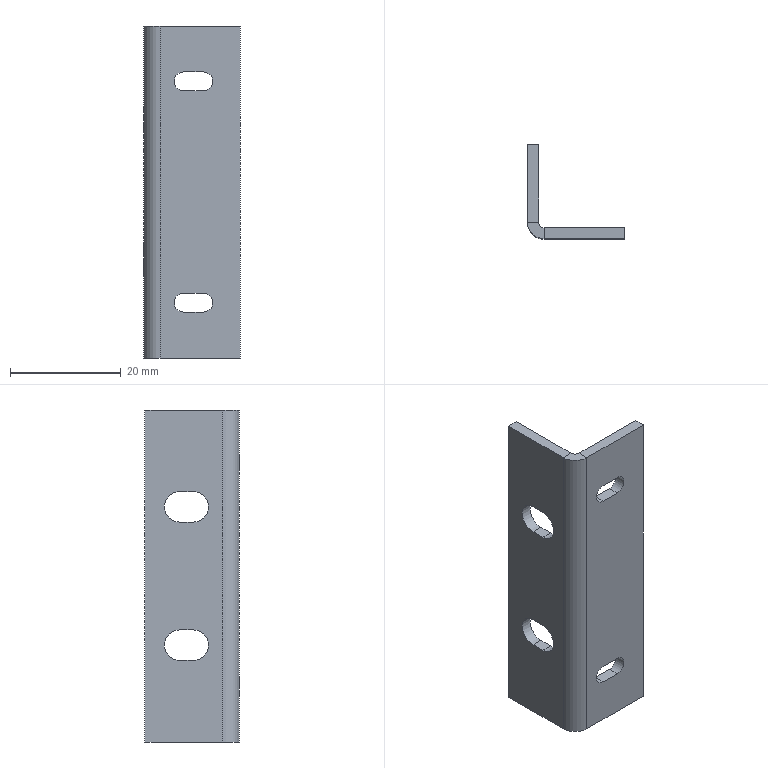Part | SolidWorks | features HoleWzd 2, FlatPattern 1, SMBaseFlange 1, SheetMetal 1 | 1 solid | 30 faces | box 17.5 x 17 x 60 mm | volume 3562 mm3 | plane 20 | cylinder 10 | commonest cylinder face diameters 3.4 x4 5.5 x4 2 x1 6 x1
STEP:
#1=CARTESIAN_POINT('',(0.,-14.,60.));
#2=VERTEX_POINT('',#1);
#3=CARTESIAN_POINT('',(2.,-14.,60.));
#4=VERTEX_POINT('',#3);
#5=CARTESIAN_POINT('',(0.,-14.,60.));
#6=DIRECTION('',(1.,0.,0.));
#7=VECTOR('',#6,1000.);
#8=LINE('',#5,#7);
#9=EDGE_CURVE('',#2,#4,#8,.T.);
#10=ORIENTED_EDGE('',*,*,#9,.F.);
#11=CARTESIAN_POINT('',(3.,-17.,60.));
#12=VERTEX_POINT('',#11);
#13=CARTESIAN_POINT('',(3.,-14.,60.));
#14=DIRECTION('',(0.,0.,1.));
#15=DIRECTION('',(-1.,0.,0.));
#16=AXIS2_PLACEMENT_3D('',#13,#14,#15);
#17=CIRCLE('',#16,3.);
#18=EDGE_CURVE('',#2,#12,#17,.T.);
#19=ORIENTED_EDGE('',*,*,#18,.T.);
#20=CARTESIAN_POINT('',(3.,-15.,60.));
#21=VERTEX_POINT('',#20);
#22=CARTESIAN_POINT('',(3.,-15.,60.));
#23=DIRECTION('',(0.,-1.,0.));
#24=VECTOR('',#23,1000.);
#25=LINE('',#22,#24);
#26=EDGE_CURVE('',#21,#12,#25,.T.);
#27=ORIENTED_EDGE('',*,*,#26,.F.);
#28=CARTESIAN_POINT('',(3.,-14.,60.));
#29=DIRECTION('',(0.,0.,1.));
#30=DIRECTION('',(1.,0.,0.));
#31=AXIS2_PLACEMENT_3D('',#28,#29,#30);
#32=CIRCLE('',#31,1.);
#33=EDGE_CURVE('',#4,#21,#32,.T.);
#34=ORIENTED_EDGE('',*,*,#33,.F.);
#35=EDGE_LOOP('',(#10,#19,#27,#34));
#36=FACE_OUTER_BOUND('',#35,.T.);
#37=CARTESIAN_POINT('',(0.,-14.,60.));
#38=DIRECTION('',(0.,0.,1.));
#39=DIRECTION('',(1.,0.,0.));
#40=AXIS2_PLACEMENT_3D('',#37,#38,#39);
#41=PLANE('',#40);
#42=ADVANCED_FACE('',(#36),#41,.T.);
#43=CARTESIAN_POINT('',(0.,0.,60.));
#44=VERTEX_POINT('',#43);
#45=CARTESIAN_POINT('',(0.,0.,60.));
#46=DIRECTION('',(0.,-1.,0.));
#47=VECTOR('',#46,1000.);
#48=LINE('',#45,#47);
#49=EDGE_CURVE('',#44,#2,#48,.T.);
#50=ORIENTED_EDGE('',*,*,#49,.T.);
#51=ORIENTED_EDGE('',*,*,#9,.T.);
#52=CARTESIAN_POINT('',(2.,0.,60.));
#53=VERTEX_POINT('',#52);
#54=CARTESIAN_POINT('',(2.,0.,60.));
#55=DIRECTION('',(0.,-1.,0.));
#56=VECTOR('',#55,1000.);
#57=LINE('',#54,#56);
#58=EDGE_CURVE('',#53,#4,#57,.T.);
#59=ORIENTED_EDGE('',*,*,#58,.F.);
#60=CARTESIAN_POINT('',(0.,0.,60.));
#61=DIRECTION('',(1.,0.,0.));
#62=VECTOR('',#61,1000.);
#63=LINE('',#60,#62);
#64=EDGE_CURVE('',#44,#53,#63,.T.);
#65=ORIENTED_EDGE('',*,*,#64,.F.);
#66=EDGE_LOOP('',(#50,#51,#59,#65));
#67=FACE_OUTER_BOUND('',#66,.T.);
#68=CARTESIAN_POINT('',(3.,-15.,60.));
#69=DIRECTION('',(0.,0.,1.));
#70=DIRECTION('',(1.,0.,0.));
#71=AXIS2_PLACEMENT_3D('',#68,#69,#70);
#72=PLANE('',#71);
#73=ADVANCED_FACE('',(#67),#72,.T.);
#74=CARTESIAN_POINT('',(3.,-17.,0.));
#75=VERTEX_POINT('',#74);
#76=CARTESIAN_POINT('',(3.,-15.,0.));
#77=VERTEX_POINT('',#76);
#78=CARTESIAN_POINT('',(3.,-17.,0.));
#79=DIRECTION('',(0.,1.,0.));
#80=VECTOR('',#79,1000.);
#81=LINE('',#78,#80);
#82=EDGE_CURVE('',#75,#77,#81,.T.);
#83=ORIENTED_EDGE('',*,*,#82,.F.);
#84=CARTESIAN_POINT('',(0.,-14.,0.));
#85=VERTEX_POINT('',#84);
#86=CARTESIAN_POINT('',(3.,-14.,0.));
#87=DIRECTION('',(0.,0.,1.));
#88=DIRECTION('',(-1.,0.,0.));
#89=AXIS2_PLACEMENT_3D('',#86,#87,#88);
#90=CIRCLE('',#89,3.);
#91=EDGE_CURVE('',#85,#75,#90,.T.);
#92=ORIENTED_EDGE('',*,*,#91,.F.);
#93=CARTESIAN_POINT('',(2.,-14.,0.));
#94=VERTEX_POINT('',#93);
#95=CARTESIAN_POINT('',(2.,-14.,0.));
#96=DIRECTION('',(-1.,0.,0.));
#97=VECTOR('',#96,1000.);
#98=LINE('',#95,#97);
#99=EDGE_CURVE('',#94,#85,#98,.T.);
#100=ORIENTED_EDGE('',*,*,#99,.F.);
#101=CARTESIAN_POINT('',(3.,-14.,0.));
#102=DIRECTION('',(0.,0.,1.));
#103=DIRECTION('',(1.,0.,0.));
#104=AXIS2_PLACEMENT_3D('',#101,#102,#103);
#105=CIRCLE('',#104,1.);
#106=EDGE_CURVE('',#94,#77,#105,.T.);
#107=ORIENTED_EDGE('',*,*,#106,.T.);
#108=EDGE_LOOP('',(#83,#92,#100,#107));
#109=FACE_OUTER_BOUND('',#108,.T.);
#110=CARTESIAN_POINT('',(3.,-17.,0.));
#111=DIRECTION('',(0.,0.,-1.));
#112=DIRECTION('',(-1.,0.,0.));
#113=AXIS2_PLACEMENT_3D('',#110,#111,#112);
#114=PLANE('',#113);
#115=ADVANCED_FACE('',(#109),#114,.T.);
#116=CARTESIAN_POINT('',(17.5,-17.,0.));
#117=VERTEX_POINT('',#116);
#118=CARTESIAN_POINT('',(0.,-17.,0.));
#119=DIRECTION('',(1.,0.,0.));
#120=VECTOR('',#119,1000.);
#121=LINE('',#118,#120);
#122=EDGE_CURVE('',#75,#117,#121,.T.);
#123=ORIENTED_EDGE('',*,*,#122,.F.);
#124=ORIENTED_EDGE('',*,*,#82,.T.);
#125=CARTESIAN_POINT('',(17.5,-15.,0.));
#126=VERTEX_POINT('',#125);
#127=CARTESIAN_POINT('',(0.,-15.,0.));
#128=DIRECTION('',(1.,0.,0.));
#129=VECTOR('',#128,1000.);
#130=LINE('',#127,#129);
#131=EDGE_CURVE('',#77,#126,#130,.T.);
#132=ORIENTED_EDGE('',*,*,#131,.T.);
#133=CARTESIAN_POINT('',(17.5,-15.,0.));
#134=DIRECTION('',(0.,-1.,0.));
#135=VECTOR('',#134,1000.);
#136=LINE('',#133,#135);
#137=EDGE_CURVE('',#126,#117,#136,.T.);
#138=ORIENTED_EDGE('',*,*,#137,.T.);
#139=EDGE_LOOP('',(#123,#124,#132,#138));
#140=FACE_OUTER_BOUND('',#139,.T.);
#141=CARTESIAN_POINT('',(2.,-14.,0.));
#142=DIRECTION('',(0.,0.,-1.));
#143=DIRECTION('',(-1.,0.,0.));
#144=AXIS2_PLACEMENT_3D('',#141,#142,#143);
#145=PLANE('',#144);
#146=ADVANCED_FACE('',(#140),#145,.T.);
#147=CARTESIAN_POINT('',(10.8,-17.,8.3));
#148=VERTEX_POINT('',#147);
#149=CARTESIAN_POINT('',(7.2,-17.,8.3));
#150=VERTEX_POINT('',#149);
#151=CARTESIAN_POINT('',(0.,-17.,8.3));
#152=DIRECTION('',(-1.,0.,0.));
#153=VECTOR('',#152,1000.);
#154=LINE('',#151,#153);
#155=EDGE_CURVE('',#148,#150,#154,.T.);
#156=ORIENTED_EDGE('',*,*,#155,.T.);
#157=CARTESIAN_POINT('',(7.2,-17.,11.7));
#158=VERTEX_POINT('',#157);
#159=CARTESIAN_POINT('',(7.2,-17.,10.));
#160=DIRECTION('',(0.,1.,0.));
#161=DIRECTION('',(0.,0.,1.));
#162=AXIS2_PLACEMENT_3D('',#159,#160,#161);
#163=CIRCLE('',#162,1.7);
#164=EDGE_CURVE('',#150,#158,#163,.T.);
#165=ORIENTED_EDGE('',*,*,#164,.T.);
#166=CARTESIAN_POINT('',(10.8,-17.,11.7));
#167=VERTEX_POINT('',#166);
#168=CARTESIAN_POINT('',(0.,-17.,11.7));
#169=DIRECTION('',(1.,0.,0.));
#170=VECTOR('',#169,1000.);
#171=LINE('',#168,#170);
#172=EDGE_CURVE('',#158,#167,#171,.T.);
#173=ORIENTED_EDGE('',*,*,#172,.T.);
#174=CARTESIAN_POINT('',(10.8,-17.,10.));
#175=DIRECTION('',(0.,1.,0.));
#176=DIRECTION('',(0.,0.,1.));
#177=AXIS2_PLACEMENT_3D('',#174,#175,#176);
#178=CIRCLE('',#177,1.7);
#179=EDGE_CURVE('',#167,#148,#178,.T.);
#180=ORIENTED_EDGE('',*,*,#179,.T.);
#181=EDGE_LOOP('',(#156,#165,#173,#180));
#182=FACE_BOUND('',#181,.T.);
#183=CARTESIAN_POINT('',(10.8,-17.,48.3));
#184=VERTEX_POINT('',#183);
#185=CARTESIAN_POINT('',(7.2,-17.,48.3));
#186=VERTEX_POINT('',#185);
#187=CARTESIAN_POINT('',(0.,-17.,48.3));
#188=DIRECTION('',(-1.,0.,0.));
#189=VECTOR('',#188,1000.);
#190=LINE('',#187,#189);
#191=EDGE_CURVE('',#184,#186,#190,.T.);
#192=ORIENTED_EDGE('',*,*,#191,.T.);
#193=CARTESIAN_POINT('',(7.2,-17.,51.7));
#194=VERTEX_POINT('',#193);
#195=CARTESIAN_POINT('',(7.2,-17.,50.));
#196=DIRECTION('',(0.,1.,0.));
#197=DIRECTION('',(0.,0.,1.));
#198=AXIS2_PLACEMENT_3D('',#195,#196,#197);
#199=CIRCLE('',#198,1.7);
#200=EDGE_CURVE('',#186,#194,#199,.T.);
#201=ORIENTED_EDGE('',*,*,#200,.T.);
#202=CARTESIAN_POINT('',(10.8,-17.,51.7));
#203=VERTEX_POINT('',#202);
#204=CARTESIAN_POINT('',(0.,-17.,51.7));
#205=DIRECTION('',(1.,0.,0.));
#206=VECTOR('',#205,1000.);
#207=LINE('',#204,#206);
#208=EDGE_CURVE('',#194,#203,#207,.T.);
#209=ORIENTED_EDGE('',*,*,#208,.T.);
#210=CARTESIAN_POINT('',(10.8,-17.,50.));
#211=DIRECTION('',(0.,1.,0.));
#212=DIRECTION('',(0.,0.,1.));
#213=AXIS2_PLACEMENT_3D('',#210,#211,#212);
#214=CIRCLE('',#213,1.7);
#215=EDGE_CURVE('',#203,#184,#214,.T.);
#216=ORIENTED_EDGE('',*,*,#215,.T.);
#217=EDGE_LOOP('',(#192,#201,#209,#216));
#218=FACE_BOUND('',#217,.T.);
#219=ORIENTED_EDGE('',*,*,#122,.T.);
#220=CARTESIAN_POINT('',(17.5,-17.,60.));
#221=VERTEX_POINT('',#220);
#222=CARTESIAN_POINT('',(17.5,-17.,60.));
#223=DIRECTION('',(0.,0.,-1.));
#224=VECTOR('',#223,1000.);
#225=LINE('',#222,#224);
#226=EDGE_CURVE('',#221,#117,#225,.T.);
#227=ORIENTED_EDGE('',*,*,#226,.F.);
#228=CARTESIAN_POINT('',(0.,-17.,60.));
#229=DIRECTION('',(1.,0.,0.));
#230=VECTOR('',#229,1000.);
#231=LINE('',#228,#230);
#232=EDGE_CURVE('',#12,#221,#231,.T.);
#233=ORIENTED_EDGE('',*,*,#232,.F.);
#234=CARTESIAN_POINT('',(3.,-17.,60.));
#235=DIRECTION('',(0.,0.,-1.));
#236=VECTOR('',#235,1000.);
#237=LINE('',#234,#236);
#238=EDGE_CURVE('',#12,#75,#237,.T.);
#239=ORIENTED_EDGE('',*,*,#238,.T.);
#240=EDGE_LOOP('',(#219,#227,#233,#239));
#241=FACE_OUTER_BOUND('',#240,.T.);
#242=CARTESIAN_POINT('',(0.,-17.,60.));
#243=DIRECTION('',(0.,1.,0.));
#244=DIRECTION('',(0.,0.,1.));
#245=AXIS2_PLACEMENT_3D('',#242,#243,#244);
#246=PLANE('',#245);
#247=ADVANCED_FACE('',(#182,#218,#241),#246,.F.);
#248=ORIENTED_EDGE('',*,*,#137,.F.);
#249=CARTESIAN_POINT('',(17.5,-15.,60.));
#250=VERTEX_POINT('',#249);
#251=CARTESIAN_POINT('',(17.5,-15.,60.));
#252=DIRECTION('',(0.,0.,-1.));
#253=VECTOR('',#252,1000.);
#254=LINE('',#251,#253);
#255=EDGE_CURVE('',#250,#126,#254,.T.);
#256=ORIENTED_EDGE('',*,*,#255,.F.);
#257=CARTESIAN_POINT('',(17.5,-15.,60.));
#258=DIRECTION('',(0.,-1.,0.));
#259=VECTOR('',#258,1000.);
#260=LINE('',#257,#259);
#261=EDGE_CURVE('',#250,#221,#260,.T.);
#262=ORIENTED_EDGE('',*,*,#261,.T.);
#263=ORIENTED_EDGE('',*,*,#226,.T.);
#264=EDGE_LOOP('',(#248,#256,#262,#263));
#265=FACE_OUTER_BOUND('',#264,.T.);
#266=CARTESIAN_POINT('',(17.5,-15.,60.));
#267=DIRECTION('',(1.,0.,0.));
#268=DIRECTION('',(0.,0.,-1.));
#269=AXIS2_PLACEMENT_3D('',#266,#267,#268);
#270=PLANE('',#269);
#271=ADVANCED_FACE('',(#265),#270,.T.);
#272=CARTESIAN_POINT('',(10.8,-15.,11.7));
#273=VERTEX_POINT('',#272);
#274=CARTESIAN_POINT('',(10.8,-15.,8.3));
#275=VERTEX_POINT('',#274);
#276=CARTESIAN_POINT('',(10.8,-15.,10.));
#277=DIRECTION('',(0.,1.,0.));
#278=DIRECTION('',(0.,0.,1.));
#279=AXIS2_PLACEMENT_3D('',#276,#277,#278);
#280=CIRCLE('',#279,1.7);
#281=EDGE_CURVE('',#273,#275,#280,.T.);
#282=ORIENTED_EDGE('',*,*,#281,.F.);
#283=CARTESIAN_POINT('',(7.2,-15.,11.7));
#284=VERTEX_POINT('',#283);
#285=CARTESIAN_POINT('',(7.2,-15.,11.7));
#286=DIRECTION('',(1.,0.,0.));
#287=VECTOR('',#286,1000.);
#288=LINE('',#285,#287);
#289=EDGE_CURVE('',#284,#273,#288,.T.);
#290=ORIENTED_EDGE('',*,*,#289,.F.);
#291=CARTESIAN_POINT('',(7.2,-15.,8.3));
#292=VERTEX_POINT('',#291);
#293=CARTESIAN_POINT('',(7.2,-15.,10.));
#294=DIRECTION('',(0.,1.,0.));
#295=DIRECTION('',(0.,0.,1.));
#296=AXIS2_PLACEMENT_3D('',#293,#294,#295);
#297=CIRCLE('',#296,1.7);
#298=EDGE_CURVE('',#292,#284,#297,.T.);
#299=ORIENTED_EDGE('',*,*,#298,.F.);
#300=CARTESIAN_POINT('',(7.2,-15.,8.3));
#301=DIRECTION('',(1.,0.,0.));
#302=VECTOR('',#301,1000.);
#303=LINE('',#300,#302);
#304=EDGE_CURVE('',#292,#275,#303,.T.);
#305=ORIENTED_EDGE('',*,*,#304,.T.);
#306=EDGE_LOOP('',(#282,#290,#299,#305));
#307=FACE_BOUND('',#306,.T.);
#308=CARTESIAN_POINT('',(7.2,-15.,51.7));
#309=VERTEX_POINT('',#308);
#310=CARTESIAN_POINT('',(10.8,-15.,51.7));
#311=VERTEX_POINT('',#310);
#312=CARTESIAN_POINT('',(7.2,-15.,51.7));
#313=DIRECTION('',(1.,0.,0.));
#314=VECTOR('',#313,1000.);
#315=LINE('',#312,#314);
#316=EDGE_CURVE('',#309,#311,#315,.T.);
#317=ORIENTED_EDGE('',*,*,#316,.F.);
#318=CARTESIAN_POINT('',(7.2,-15.,48.3));
#319=VERTEX_POINT('',#318);
#320=CARTESIAN_POINT('',(7.2,-15.,50.));
#321=DIRECTION('',(0.,1.,0.));
#322=DIRECTION('',(0.,0.,1.));
#323=AXIS2_PLACEMENT_3D('',#320,#321,#322);
#324=CIRCLE('',#323,1.7);
#325=EDGE_CURVE('',#319,#309,#324,.T.);
#326=ORIENTED_EDGE('',*,*,#325,.F.);
#327=CARTESIAN_POINT('',(10.8,-15.,48.3));
#328=VERTEX_POINT('',#327);
#329=CARTESIAN_POINT('',(7.2,-15.,48.3));
#330=DIRECTION('',(1.,0.,0.));
#331=VECTOR('',#330,1000.);
#332=LINE('',#329,#331);
#333=EDGE_CURVE('',#319,#328,#332,.T.);
#334=ORIENTED_EDGE('',*,*,#333,.T.);
#335=CARTESIAN_POINT('',(10.8,-15.,50.));
#336=DIRECTION('',(0.,1.,0.));
#337=DIRECTION('',(0.,0.,1.));
#338=AXIS2_PLACEMENT_3D('',#335,#336,#337);
#339=CIRCLE('',#338,1.7);
#340=EDGE_CURVE('',#311,#328,#339,.T.);
#341=ORIENTED_EDGE('',*,*,#340,.F.);
#342=EDGE_LOOP('',(#317,#326,#334,#341));
#343=FACE_BOUND('',#342,.T.);
#344=ORIENTED_EDGE('',*,*,#131,.F.);
#345=CARTESIAN_POINT('',(3.,-15.,60.));
#346=DIRECTION('',(0.,0.,-1.));
#347=VECTOR('',#346,1000.);
#348=LINE('',#345,#347);
#349=EDGE_CURVE('',#21,#77,#348,.T.);
#350=ORIENTED_EDGE('',*,*,#349,.F.);
#351=CARTESIAN_POINT('',(0.,-15.,60.));
#352=DIRECTION('',(1.,0.,0.));
#353=VECTOR('',#352,1000.);
#354=LINE('',#351,#353);
#355=EDGE_CURVE('',#21,#250,#354,.T.);
#356=ORIENTED_EDGE('',*,*,#355,.T.);
#357=ORIENTED_EDGE('',*,*,#255,.T.);
#358=EDGE_LOOP('',(#344,#350,#356,#357));
#359=FACE_OUTER_BOUND('',#358,.T.);
#360=CARTESIAN_POINT('',(0.,-15.,60.));
#361=DIRECTION('',(0.,1.,0.));
#362=DIRECTION('',(0.,0.,1.));
#363=AXIS2_PLACEMENT_3D('',#360,#361,#362);
#364=PLANE('',#363);
#365=ADVANCED_FACE('',(#307,#343,#359),#364,.T.);
#366=ORIENTED_EDGE('',*,*,#106,.F.);
#367=CARTESIAN_POINT('',(2.,-14.,60.));
#368=DIRECTION('',(0.,0.,-1.));
#369=VECTOR('',#368,1000.);
#370=LINE('',#367,#369);
#371=EDGE_CURVE('',#4,#94,#370,.T.);
#372=ORIENTED_EDGE('',*,*,#371,.F.);
#373=ORIENTED_EDGE('',*,*,#33,.T.);
#374=ORIENTED_EDGE('',*,*,#349,.T.);
#375=EDGE_LOOP('',(#366,#372,#373,#374));
#376=FACE_OUTER_BOUND('',#375,.T.);
#377=CARTESIAN_POINT('',(3.,-14.,60.));
#378=DIRECTION('',(0.,0.,-1.));
#379=DIRECTION('',(-1.,0.,0.));
#380=AXIS2_PLACEMENT_3D('',#377,#378,#379);
#381=CYLINDRICAL_SURFACE('',#380,1.);
#382=ADVANCED_FACE('',(#376),#381,.F.);
#383=CARTESIAN_POINT('',(2.,-6.25,14.75));
#384=VERTEX_POINT('',#383);
#385=CARTESIAN_POINT('',(2.,-6.25,20.25));
#386=VERTEX_POINT('',#385);
#387=CARTESIAN_POINT('',(2.,-6.25,17.5));
#388=DIRECTION('',(1.,0.,0.));
#389=DIRECTION('',(0.,0.,-1.));
#390=AXIS2_PLACEMENT_3D('',#387,#388,#389);
#391=CIRCLE('',#390,2.75);
#392=EDGE_CURVE('',#384,#386,#391,.T.);
#393=ORIENTED_EDGE('',*,*,#392,.F.);
#394=CARTESIAN_POINT('',(2.,-8.75,14.75));
#395=VERTEX_POINT('',#394);
#396=CARTESIAN_POINT('',(2.,-8.75,14.75));
#397=DIRECTION('',(0.,1.,0.));
#398=VECTOR('',#397,1000.);
#399=LINE('',#396,#398);
#400=EDGE_CURVE('',#395,#384,#399,.T.);
#401=ORIENTED_EDGE('',*,*,#400,.F.);
#402=CARTESIAN_POINT('',(2.,-8.75,20.25));
#403=VERTEX_POINT('',#402);
#404=CARTESIAN_POINT('',(2.,-8.75,17.5));
#405=DIRECTION('',(1.,0.,0.));
#406=DIRECTION('',(0.,0.,-1.));
#407=AXIS2_PLACEMENT_3D('',#404,#405,#406);
#408=CIRCLE('',#407,2.75);
#409=EDGE_CURVE('',#403,#395,#408,.T.);
#410=ORIENTED_EDGE('',*,*,#409,.F.);
#411=CARTESIAN_POINT('',(2.,-8.75,20.25));
#412=DIRECTION('',(0.,1.,0.));
#413=VECTOR('',#412,1000.);
#414=LINE('',#411,#413);
#415=EDGE_CURVE('',#403,#386,#414,.T.);
#416=ORIENTED_EDGE('',*,*,#415,.T.);
#417=EDGE_LOOP('',(#393,#401,#410,#416));
#418=FACE_BOUND('',#417,.T.);
#419=CARTESIAN_POINT('',(2.,-8.75,39.75));
#420=VERTEX_POINT('',#419);
#421=CARTESIAN_POINT('',(2.,-6.25,39.75));
#422=VERTEX_POINT('',#421);
#423=CARTESIAN_POINT('',(2.,-8.75,39.75));
#424=DIRECTION('',(0.,1.,0.));
#425=VECTOR('',#424,1000.);
#426=LINE('',#423,#425);
#427=EDGE_CURVE('',#420,#422,#426,.T.);
#428=ORIENTED_EDGE('',*,*,#427,.F.);
#429=CARTESIAN_POINT('',(2.,-8.75,45.25));
#430=VERTEX_POINT('',#429);
#431=CARTESIAN_POINT('',(2.,-8.75,42.5));
#432=DIRECTION('',(1.,0.,0.));
#433=DIRECTION('',(0.,0.,-1.));
#434=AXIS2_PLACEMENT_3D('',#431,#432,#433);
#435=CIRCLE('',#434,2.75);
#436=EDGE_CURVE('',#430,#420,#435,.T.);
#437=ORIENTED_EDGE('',*,*,#436,.F.);
#438=CARTESIAN_POINT('',(2.,-6.25,45.25));
#439=VERTEX_POINT('',#438);
#440=CARTESIAN_POINT('',(2.,-8.75,45.25));
#441=DIRECTION('',(0.,1.,0.));
#442=VECTOR('',#441,1000.);
#443=LINE('',#440,#442);
#444=EDGE_CURVE('',#430,#439,#443,.T.);
#445=ORIENTED_EDGE('',*,*,#444,.T.);
#446=CARTESIAN_POINT('',(2.,-6.25,42.5));
#447=DIRECTION('',(1.,0.,0.));
#448=DIRECTION('',(0.,0.,-1.));
#449=AXIS2_PLACEMENT_3D('',#446,#447,#448);
#450=CIRCLE('',#449,2.75);
#451=EDGE_CURVE('',#422,#439,#450,.T.);
#452=ORIENTED_EDGE('',*,*,#451,.F.);
#453=EDGE_LOOP('',(#428,#437,#445,#452));
#454=FACE_BOUND('',#453,.T.);
#455=CARTESIAN_POINT('',(2.,0.,0.));
#456=VERTEX_POINT('',#455);
#457=CARTESIAN_POINT('',(2.,0.,0.));
#458=DIRECTION('',(0.,-1.,0.));
#459=VECTOR('',#458,1000.);
#460=LINE('',#457,#459);
#461=EDGE_CURVE('',#456,#94,#460,.T.);
#462=ORIENTED_EDGE('',*,*,#461,.F.);
#463=CARTESIAN_POINT('',(2.,0.,60.));
#464=DIRECTION('',(0.,0.,-1.));
#465=VECTOR('',#464,1000.);
#466=LINE('',#463,#465);
#467=EDGE_CURVE('',#53,#456,#466,.T.);
#468=ORIENTED_EDGE('',*,*,#467,.F.);
#469=ORIENTED_EDGE('',*,*,#58,.T.);
#470=ORIENTED_EDGE('',*,*,#371,.T.);
#471=EDGE_LOOP('',(#462,#468,#469,#470));
#472=FACE_OUTER_BOUND('',#471,.T.);
#473=CARTESIAN_POINT('',(2.,0.,60.));
#474=DIRECTION('',(1.,0.,0.));
#475=DIRECTION('',(0.,1.,0.));
#476=AXIS2_PLACEMENT_3D('',#473,#474,#475);
#477=PLANE('',#476);
#478=ADVANCED_FACE('',(#418,#454,#472),#477,.T.);
#479=CARTESIAN_POINT('',(0.,0.,0.));
#480=VERTEX_POINT('',#479);
#481=CARTESIAN_POINT('',(0.,0.,0.));
#482=DIRECTION('',(1.,0.,0.));
#483=VECTOR('',#482,1000.);
#484=LINE('',#481,#483);
#485=EDGE_CURVE('',#480,#456,#484,.T.);
#486=ORIENTED_EDGE('',*,*,#485,.F.);
#487=CARTESIAN_POINT('',(0.,0.,60.));
#488=DIRECTION('',(0.,0.,-1.));
#489=VECTOR('',#488,1000.);
#490=LINE('',#487,#489);
#491=EDGE_CURVE('',#44,#480,#490,.T.);
#492=ORIENTED_EDGE('',*,*,#491,.F.);
#493=ORIENTED_EDGE('',*,*,#64,.T.);
#494=ORIENTED_EDGE('',*,*,#467,.T.);
#495=EDGE_LOOP('',(#486,#492,#493,#494));
#496=FACE_OUTER_BOUND('',#495,.T.);
#497=CARTESIAN_POINT('',(0.,0.,60.));
#498=DIRECTION('',(0.,1.,0.));
#499=DIRECTION('',(-1.,0.,0.));
#500=AXIS2_PLACEMENT_3D('',#497,#498,#499);
#501=PLANE('',#500);
#502=ADVANCED_FACE('',(#496),#501,.T.);
#503=CARTESIAN_POINT('',(0.,-6.25,20.25));
#504=VERTEX_POINT('',#503);
#505=CARTESIAN_POINT('',(0.,-8.75,20.25));
#506=VERTEX_POINT('',#505);
#507=CARTESIAN_POINT('',(0.,0.,20.25));
#508=DIRECTION('',(0.,-1.,0.));
#509=VECTOR('',#508,1000.);
#510=LINE('',#507,#509);
#511=EDGE_CURVE('',#504,#506,#510,.T.);
#512=ORIENTED_EDGE('',*,*,#511,.T.);
#513=CARTESIAN_POINT('',(0.,-8.75,14.75));
#514=VERTEX_POINT('',#513);
#515=CARTESIAN_POINT('',(0.,-8.75,17.5));
#516=DIRECTION('',(1.,0.,0.));
#517=DIRECTION('',(0.,1.,0.));
#518=AXIS2_PLACEMENT_3D('',#515,#516,#517);
#519=CIRCLE('',#518,2.75);
#520=EDGE_CURVE('',#506,#514,#519,.T.);
#521=ORIENTED_EDGE('',*,*,#520,.T.);
#522=CARTESIAN_POINT('',(0.,-6.25,14.75));
#523=VERTEX_POINT('',#522);
#524=CARTESIAN_POINT('',(0.,0.,14.75));
#525=DIRECTION('',(0.,1.,0.));
#526=VECTOR('',#525,1000.);
#527=LINE('',#524,#526);
#528=EDGE_CURVE('',#514,#523,#527,.T.);
#529=ORIENTED_EDGE('',*,*,#528,.T.);
#530=CARTESIAN_POINT('',(0.,-6.25,17.5));
#531=DIRECTION('',(1.,0.,0.));
#532=DIRECTION('',(0.,1.,0.));
#533=AXIS2_PLACEMENT_3D('',#530,#531,#532);
#534=CIRCLE('',#533,2.75);
#535=EDGE_CURVE('',#523,#504,#534,.T.);
#536=ORIENTED_EDGE('',*,*,#535,.T.);
#537=EDGE_LOOP('',(#512,#521,#529,#536));
#538=FACE_BOUND('',#537,.T.);
#539=CARTESIAN_POINT('',(0.,-8.75,39.75));
#540=VERTEX_POINT('',#539);
#541=CARTESIAN_POINT('',(0.,-6.25,39.75));
#542=VERTEX_POINT('',#541);
#543=CARTESIAN_POINT('',(0.,0.,39.75));
#544=DIRECTION('',(0.,1.,0.));
#545=VECTOR('',#544,1000.);
#546=LINE('',#543,#545);
#547=EDGE_CURVE('',#540,#542,#546,.T.);
#548=ORIENTED_EDGE('',*,*,#547,.T.);
#549=CARTESIAN_POINT('',(0.,-6.25,45.25));
#550=VERTEX_POINT('',#549);
#551=CARTESIAN_POINT('',(0.,-6.25,42.5));
#552=DIRECTION('',(1.,0.,0.));
#553=DIRECTION('',(0.,1.,0.));
#554=AXIS2_PLACEMENT_3D('',#551,#552,#553);
#555=CIRCLE('',#554,2.75);
#556=EDGE_CURVE('',#542,#550,#555,.T.);
#557=ORIENTED_EDGE('',*,*,#556,.T.);
#558=CARTESIAN_POINT('',(0.,-8.75,45.25));
#559=VERTEX_POINT('',#558);
#560=CARTESIAN_POINT('',(0.,0.,45.25));
#561=DIRECTION('',(0.,-1.,0.));
#562=VECTOR('',#561,1000.);
#563=LINE('',#560,#562);
#564=EDGE_CURVE('',#550,#559,#563,.T.);
#565=ORIENTED_EDGE('',*,*,#564,.T.);
#566=CARTESIAN_POINT('',(0.,-8.75,42.5));
#567=DIRECTION('',(1.,0.,0.));
#568=DIRECTION('',(0.,1.,0.));
#569=AXIS2_PLACEMENT_3D('',#566,#567,#568);
#570=CIRCLE('',#569,2.75);
#571=EDGE_CURVE('',#559,#540,#570,.T.);
#572=ORIENTED_EDGE('',*,*,#571,.T.);
#573=EDGE_LOOP('',(#548,#557,#565,#572));
#574=FACE_BOUND('',#573,.T.);
#575=CARTESIAN_POINT('',(0.,0.,0.));
#576=DIRECTION('',(0.,-1.,0.));
#577=VECTOR('',#576,1000.);
#578=LINE('',#575,#577);
#579=EDGE_CURVE('',#480,#85,#578,.T.);
#580=ORIENTED_EDGE('',*,*,#579,.T.);
#581=CARTESIAN_POINT('',(0.,-14.,60.));
#582=DIRECTION('',(0.,0.,-1.));
#583=VECTOR('',#582,1000.);
#584=LINE('',#581,#583);
#585=EDGE_CURVE('',#2,#85,#584,.T.);
#586=ORIENTED_EDGE('',*,*,#585,.F.);
#587=ORIENTED_EDGE('',*,*,#49,.F.);
#588=ORIENTED_EDGE('',*,*,#491,.T.);
#589=EDGE_LOOP('',(#580,#586,#587,#588));
#590=FACE_OUTER_BOUND('',#589,.T.);
#591=CARTESIAN_POINT('',(0.,0.,60.));
#592=DIRECTION('',(1.,0.,0.));
#593=DIRECTION('',(0.,1.,0.));
#594=AXIS2_PLACEMENT_3D('',#591,#592,#593);
#595=PLANE('',#594);
#596=ADVANCED_FACE('',(#538,#574,#590),#595,.F.);
#597=ORIENTED_EDGE('',*,*,#91,.T.);
#598=ORIENTED_EDGE('',*,*,#238,.F.);
#599=ORIENTED_EDGE('',*,*,#18,.F.);
#600=ORIENTED_EDGE('',*,*,#585,.T.);
#601=EDGE_LOOP('',(#597,#598,#599,#600));
#602=FACE_OUTER_BOUND('',#601,.T.);
#603=CARTESIAN_POINT('',(3.,-14.,60.));
#604=DIRECTION('',(0.,0.,-1.));
#605=DIRECTION('',(-1.,0.,0.));
#606=AXIS2_PLACEMENT_3D('',#603,#604,#605);
#607=CYLINDRICAL_SURFACE('',#606,3.);
#608=ADVANCED_FACE('',(#602),#607,.T.);
#609=ORIENTED_EDGE('',*,*,#232,.T.);
#610=ORIENTED_EDGE('',*,*,#261,.F.);
#611=ORIENTED_EDGE('',*,*,#355,.F.);
#612=ORIENTED_EDGE('',*,*,#26,.T.);
#613=EDGE_LOOP('',(#609,#610,#611,#612));
#614=FACE_OUTER_BOUND('',#613,.T.);
#615=CARTESIAN_POINT('',(3.,-14.,60.));
#616=DIRECTION('',(0.,0.,1.));
#617=DIRECTION('',(1.,0.,0.));
#618=AXIS2_PLACEMENT_3D('',#615,#616,#617);
#619=PLANE('',#618);
#620=ADVANCED_FACE('',(#614),#619,.T.);
#621=ORIENTED_EDGE('',*,*,#461,.T.);
#622=ORIENTED_EDGE('',*,*,#99,.T.);
#623=ORIENTED_EDGE('',*,*,#579,.F.);
#624=ORIENTED_EDGE('',*,*,#485,.T.);
#625=EDGE_LOOP('',(#621,#622,#623,#624));
#626=FACE_OUTER_BOUND('',#625,.T.);
#627=CARTESIAN_POINT('',(3.,-14.,0.));
#628=DIRECTION('',(0.,0.,1.));
#629=DIRECTION('',(1.,0.,0.));
#630=AXIS2_PLACEMENT_3D('',#627,#628,#629);
#631=PLANE('',#630);
#632=ADVANCED_FACE('',(#626),#631,.F.);
#633=CARTESIAN_POINT('',(7.2,-15.,48.3));
#634=DIRECTION('',(0.,-1.,0.));
#635=VECTOR('',#634,1000.);
#636=LINE('',#633,#635);
#637=EDGE_CURVE('',#319,#186,#636,.T.);
#638=ORIENTED_EDGE('',*,*,#637,.F.);
#639=ORIENTED_EDGE('',*,*,#325,.T.);
#640=CARTESIAN_POINT('',(7.2,-15.,51.7));
#641=DIRECTION('',(0.,1.,0.));
#642=VECTOR('',#641,1000.);
#643=LINE('',#640,#642);
#644=EDGE_CURVE('',#194,#309,#643,.T.);
#645=ORIENTED_EDGE('',*,*,#644,.F.);
#646=ORIENTED_EDGE('',*,*,#200,.F.);
#647=EDGE_LOOP('',(#638,#639,#645,#646));
#648=FACE_OUTER_BOUND('',#647,.T.);
#649=CARTESIAN_POINT('',(7.2,-15.,50.));
#650=DIRECTION('',(0.,1.,0.));
#651=DIRECTION('',(0.,0.,1.));
#652=AXIS2_PLACEMENT_3D('',#649,#650,#651);
#653=CYLINDRICAL_SURFACE('',#652,1.7);
#654=ADVANCED_FACE('',(#648),#653,.F.);
#655=ORIENTED_EDGE('',*,*,#644,.T.);
#656=ORIENTED_EDGE('',*,*,#316,.T.);
#657=CARTESIAN_POINT('',(10.8,-15.,51.7));
#658=DIRECTION('',(0.,-1.,0.));
#659=VECTOR('',#658,1000.);
#660=LINE('',#657,#659);
#661=EDGE_CURVE('',#311,#203,#660,.T.);
#662=ORIENTED_EDGE('',*,*,#661,.T.);
#663=ORIENTED_EDGE('',*,*,#208,.F.);
#664=EDGE_LOOP('',(#655,#656,#662,#663));
#665=FACE_OUTER_BOUND('',#664,.T.);
#666=CARTESIAN_POINT('',(7.2,-15.,51.7));
#667=DIRECTION('',(0.,0.,1.));
#668=DIRECTION('',(1.,0.,0.));
#669=AXIS2_PLACEMENT_3D('',#666,#667,#668);
#670=PLANE('',#669);
#671=ADVANCED_FACE('',(#665),#670,.F.);
#672=CARTESIAN_POINT('',(10.8,-15.,48.3));
#673=DIRECTION('',(0.,1.,0.));
#674=VECTOR('',#673,1000.);
#675=LINE('',#672,#674);
#676=EDGE_CURVE('',#184,#328,#675,.T.);
#677=ORIENTED_EDGE('',*,*,#676,.T.);
#678=ORIENTED_EDGE('',*,*,#333,.F.);
#679=ORIENTED_EDGE('',*,*,#637,.T.);
#680=ORIENTED_EDGE('',*,*,#191,.F.);
#681=EDGE_LOOP('',(#677,#678,#679,#680));
#682=FACE_OUTER_BOUND('',#681,.T.);
#683=CARTESIAN_POINT('',(7.2,-15.,48.3));
#684=DIRECTION('',(0.,0.,-1.));
#685=DIRECTION('',(-1.,0.,0.));
#686=AXIS2_PLACEMENT_3D('',#683,#684,#685);
#687=PLANE('',#686);
#688=ADVANCED_FACE('',(#682),#687,.F.);
#689=ORIENTED_EDGE('',*,*,#661,.F.);
#690=ORIENTED_EDGE('',*,*,#340,.T.);
#691=ORIENTED_EDGE('',*,*,#676,.F.);
#692=ORIENTED_EDGE('',*,*,#215,.F.);
#693=EDGE_LOOP('',(#689,#690,#691,#692));
#694=FACE_OUTER_BOUND('',#693,.T.);
#695=CARTESIAN_POINT('',(10.8,-15.,50.));
#696=DIRECTION('',(0.,1.,0.));
#697=DIRECTION('',(0.,0.,1.));
#698=AXIS2_PLACEMENT_3D('',#695,#696,#697);
#699=CYLINDRICAL_SURFACE('',#698,1.7);
#700=ADVANCED_FACE('',(#694),#699,.F.);
#701=CARTESIAN_POINT('',(7.2,-15.,8.3));
#702=DIRECTION('',(0.,-1.,0.));
#703=VECTOR('',#702,1000.);
#704=LINE('',#701,#703);
#705=EDGE_CURVE('',#292,#150,#704,.T.);
#706=ORIENTED_EDGE('',*,*,#705,.F.);
#707=ORIENTED_EDGE('',*,*,#298,.T.);
#708=CARTESIAN_POINT('',(7.2,-15.,11.7));
#709=DIRECTION('',(0.,1.,0.));
#710=VECTOR('',#709,1000.);
#711=LINE('',#708,#710);
#712=EDGE_CURVE('',#158,#284,#711,.T.);
#713=ORIENTED_EDGE('',*,*,#712,.F.);
#714=ORIENTED_EDGE('',*,*,#164,.F.);
#715=EDGE_LOOP('',(#706,#707,#713,#714));
#716=FACE_OUTER_BOUND('',#715,.T.);
#717=CARTESIAN_POINT('',(7.2,-15.,10.));
#718=DIRECTION('',(0.,1.,0.));
#719=DIRECTION('',(0.,0.,1.));
#720=AXIS2_PLACEMENT_3D('',#717,#718,#719);
#721=CYLINDRICAL_SURFACE('',#720,1.7);
#722=ADVANCED_FACE('',(#716),#721,.F.);
#723=ORIENTED_EDGE('',*,*,#712,.T.);
#724=ORIENTED_EDGE('',*,*,#289,.T.);
#725=CARTESIAN_POINT('',(10.8,-15.,11.7));
#726=DIRECTION('',(0.,-1.,0.));
#727=VECTOR('',#726,1000.);
#728=LINE('',#725,#727);
#729=EDGE_CURVE('',#273,#167,#728,.T.);
#730=ORIENTED_EDGE('',*,*,#729,.T.);
#731=ORIENTED_EDGE('',*,*,#172,.F.);
#732=EDGE_LOOP('',(#723,#724,#730,#731));
#733=FACE_OUTER_BOUND('',#732,.T.);
#734=CARTESIAN_POINT('',(7.2,-15.,11.7));
#735=DIRECTION('',(0.,0.,1.));
#736=DIRECTION('',(1.,0.,0.));
#737=AXIS2_PLACEMENT_3D('',#734,#735,#736);
#738=PLANE('',#737);
#739=ADVANCED_FACE('',(#733),#738,.F.);
#740=ORIENTED_EDGE('',*,*,#729,.F.);
#741=ORIENTED_EDGE('',*,*,#281,.T.);
#742=CARTESIAN_POINT('',(10.8,-15.,8.3));
#743=DIRECTION('',(0.,1.,0.));
#744=VECTOR('',#743,1000.);
#745=LINE('',#742,#744);
#746=EDGE_CURVE('',#148,#275,#745,.T.);
#747=ORIENTED_EDGE('',*,*,#746,.F.);
#748=ORIENTED_EDGE('',*,*,#179,.F.);
#749=EDGE_LOOP('',(#740,#741,#747,#748));
#750=FACE_OUTER_BOUND('',#749,.T.);
#751=CARTESIAN_POINT('',(10.8,-15.,10.));
#752=DIRECTION('',(0.,1.,0.));
#753=DIRECTION('',(0.,0.,1.));
#754=AXIS2_PLACEMENT_3D('',#751,#752,#753);
#755=CYLINDRICAL_SURFACE('',#754,1.7);
#756=ADVANCED_FACE('',(#750),#755,.F.);
#757=ORIENTED_EDGE('',*,*,#746,.T.);
#758=ORIENTED_EDGE('',*,*,#304,.F.);
#759=ORIENTED_EDGE('',*,*,#705,.T.);
#760=ORIENTED_EDGE('',*,*,#155,.F.);
#761=EDGE_LOOP('',(#757,#758,#759,#760));
#762=FACE_OUTER_BOUND('',#761,.T.);
#763=CARTESIAN_POINT('',(7.2,-15.,8.3));
#764=DIRECTION('',(0.,0.,-1.));
#765=DIRECTION('',(-1.,0.,0.));
#766=AXIS2_PLACEMENT_3D('',#763,#764,#765);
#767=PLANE('',#766);
#768=ADVANCED_FACE('',(#762),#767,.F.);
#769=CARTESIAN_POINT('',(2.,-6.25,39.75));
#770=DIRECTION('',(-1.,0.,0.));
#771=VECTOR('',#770,1000.);
#772=LINE('',#769,#771);
#773=EDGE_CURVE('',#422,#542,#772,.T.);
#774=ORIENTED_EDGE('',*,*,#773,.F.);
#775=ORIENTED_EDGE('',*,*,#451,.T.);
#776=CARTESIAN_POINT('',(2.,-6.25,45.25));
#777=DIRECTION('',(1.,0.,0.));
#778=VECTOR('',#777,1000.);
#779=LINE('',#776,#778);
#780=EDGE_CURVE('',#550,#439,#779,.T.);
#781=ORIENTED_EDGE('',*,*,#780,.F.);
#782=ORIENTED_EDGE('',*,*,#556,.F.);
#783=EDGE_LOOP('',(#774,#775,#781,#782));
#784=FACE_OUTER_BOUND('',#783,.T.);
#785=CARTESIAN_POINT('',(2.,-6.25,42.5));
#786=DIRECTION('',(1.,0.,0.));
#787=DIRECTION('',(0.,0.,-1.));
#788=AXIS2_PLACEMENT_3D('',#785,#786,#787);
#789=CYLINDRICAL_SURFACE('',#788,2.75);
#790=ADVANCED_FACE('',(#784),#789,.F.);
#791=CARTESIAN_POINT('',(2.,-8.75,39.75));
#792=DIRECTION('',(1.,0.,0.));
#793=VECTOR('',#792,1000.);
#794=LINE('',#791,#793);
#795=EDGE_CURVE('',#540,#420,#794,.T.);
#796=ORIENTED_EDGE('',*,*,#795,.T.);
#797=ORIENTED_EDGE('',*,*,#427,.T.);
#798=ORIENTED_EDGE('',*,*,#773,.T.);
#799=ORIENTED_EDGE('',*,*,#547,.F.);
#800=EDGE_LOOP('',(#796,#797,#798,#799));
#801=FACE_OUTER_BOUND('',#800,.T.);
#802=CARTESIAN_POINT('',(2.,-8.75,39.75));
#803=DIRECTION('',(0.,0.,-1.));
#804=DIRECTION('',(-1.,0.,0.));
#805=AXIS2_PLACEMENT_3D('',#802,#803,#804);
#806=PLANE('',#805);
#807=ADVANCED_FACE('',(#801),#806,.F.);
#808=ORIENTED_EDGE('',*,*,#780,.T.);
#809=ORIENTED_EDGE('',*,*,#444,.F.);
#810=CARTESIAN_POINT('',(2.,-8.75,45.25));
#811=DIRECTION('',(-1.,0.,0.));
#812=VECTOR('',#811,1000.);
#813=LINE('',#810,#812);
#814=EDGE_CURVE('',#430,#559,#813,.T.);
#815=ORIENTED_EDGE('',*,*,#814,.T.);
#816=ORIENTED_EDGE('',*,*,#564,.F.);
#817=EDGE_LOOP('',(#808,#809,#815,#816));
#818=FACE_OUTER_BOUND('',#817,.T.);
#819=CARTESIAN_POINT('',(2.,-8.75,45.25));
#820=DIRECTION('',(0.,0.,1.));
#821=DIRECTION('',(1.,0.,0.));
#822=AXIS2_PLACEMENT_3D('',#819,#820,#821);
#823=PLANE('',#822);
#824=ADVANCED_FACE('',(#818),#823,.F.);
#825=ORIENTED_EDGE('',*,*,#814,.F.);
#826=ORIENTED_EDGE('',*,*,#436,.T.);
#827=ORIENTED_EDGE('',*,*,#795,.F.);
#828=ORIENTED_EDGE('',*,*,#571,.F.);
#829=EDGE_LOOP('',(#825,#826,#827,#828));
#830=FACE_OUTER_BOUND('',#829,.T.);
#831=CARTESIAN_POINT('',(2.,-8.75,42.5));
#832=DIRECTION('',(1.,0.,0.));
#833=DIRECTION('',(0.,0.,-1.));
#834=AXIS2_PLACEMENT_3D('',#831,#832,#833);
#835=CYLINDRICAL_SURFACE('',#834,2.75);
#836=ADVANCED_FACE('',(#830),#835,.F.);
#837=CARTESIAN_POINT('',(2.,-8.75,20.25));
#838=DIRECTION('',(-1.,0.,0.));
#839=VECTOR('',#838,1000.);
#840=LINE('',#837,#839);
#841=EDGE_CURVE('',#403,#506,#840,.T.);
#842=ORIENTED_EDGE('',*,*,#841,.F.);
#843=ORIENTED_EDGE('',*,*,#409,.T.);
#844=CARTESIAN_POINT('',(2.,-8.75,14.75));
#845=DIRECTION('',(1.,0.,0.));
#846=VECTOR('',#845,1000.);
#847=LINE('',#844,#846);
#848=EDGE_CURVE('',#514,#395,#847,.T.);
#849=ORIENTED_EDGE('',*,*,#848,.F.);
#850=ORIENTED_EDGE('',*,*,#520,.F.);
#851=EDGE_LOOP('',(#842,#843,#849,#850));
#852=FACE_OUTER_BOUND('',#851,.T.);
#853=CARTESIAN_POINT('',(2.,-8.75,17.5));
#854=DIRECTION('',(1.,0.,0.));
#855=DIRECTION('',(0.,0.,-1.));
#856=AXIS2_PLACEMENT_3D('',#853,#854,#855);
#857=CYLINDRICAL_SURFACE('',#856,2.75);
#858=ADVANCED_FACE('',(#852),#857,.F.);
#859=ORIENTED_EDGE('',*,*,#848,.T.);
#860=ORIENTED_EDGE('',*,*,#400,.T.);
#861=CARTESIAN_POINT('',(2.,-6.25,14.75));
#862=DIRECTION('',(-1.,0.,0.));
#863=VECTOR('',#862,1000.);
#864=LINE('',#861,#863);
#865=EDGE_CURVE('',#384,#523,#864,.T.);
#866=ORIENTED_EDGE('',*,*,#865,.T.);
#867=ORIENTED_EDGE('',*,*,#528,.F.);
#868=EDGE_LOOP('',(#859,#860,#866,#867));
#869=FACE_OUTER_BOUND('',#868,.T.);
#870=CARTESIAN_POINT('',(2.,-8.75,14.75));
#871=DIRECTION('',(0.,0.,-1.));
#872=DIRECTION('',(-1.,0.,0.));
#873=AXIS2_PLACEMENT_3D('',#870,#871,#872);
#874=PLANE('',#873);
#875=ADVANCED_FACE('',(#869),#874,.F.);
#876=CARTESIAN_POINT('',(2.,-6.25,20.25));
#877=DIRECTION('',(1.,0.,0.));
#878=VECTOR('',#877,1000.);
#879=LINE('',#876,#878);
#880=EDGE_CURVE('',#504,#386,#879,.T.);
#881=ORIENTED_EDGE('',*,*,#880,.T.);
#882=ORIENTED_EDGE('',*,*,#415,.F.);
#883=ORIENTED_EDGE('',*,*,#841,.T.);
#884=ORIENTED_EDGE('',*,*,#511,.F.);
#885=EDGE_LOOP('',(#881,#882,#883,#884));
#886=FACE_OUTER_BOUND('',#885,.T.);
#887=CARTESIAN_POINT('',(2.,-8.75,20.25));
#888=DIRECTION('',(0.,0.,1.));
#889=DIRECTION('',(1.,0.,0.));
#890=AXIS2_PLACEMENT_3D('',#887,#888,#889);
#891=PLANE('',#890);
#892=ADVANCED_FACE('',(#886),#891,.F.);
#893=ORIENTED_EDGE('',*,*,#865,.F.);
#894=ORIENTED_EDGE('',*,*,#392,.T.);
#895=ORIENTED_EDGE('',*,*,#880,.F.);
#896=ORIENTED_EDGE('',*,*,#535,.F.);
#897=EDGE_LOOP('',(#893,#894,#895,#896));
#898=FACE_OUTER_BOUND('',#897,.T.);
#899=CARTESIAN_POINT('',(2.,-6.25,17.5));
#900=DIRECTION('',(1.,0.,0.));
#901=DIRECTION('',(0.,0.,-1.));
#902=AXIS2_PLACEMENT_3D('',#899,#900,#901);
#903=CYLINDRICAL_SURFACE('',#902,2.75);
#904=ADVANCED_FACE('',(#898),#903,.F.);
#905=CLOSED_SHELL('',(#42,#73,#115,#146,#247,#271,#365,#382,#478,#502,#596,#608,#620,#632,#654,#671,#688,#700,#722,#739,#756,#768,#790,#807,#824,#836,#858,#875,#892,#904));
#906=MANIFOLD_SOLID_BREP('',#905);
#907=CARTESIAN_POINT('',(0.,0.,0.));
#908=DIRECTION('',(0.,0.,1.));
#909=DIRECTION('',(1.,0.,0.));
#910=AXIS2_PLACEMENT_3D('',#907,#908,#909);
#911=(LENGTH_UNIT()NAMED_UNIT(*)SI_UNIT(.MILLI.,.METRE.));
#912=UNCERTAINTY_MEASURE_WITH_UNIT(LENGTH_MEASURE(0.00001),#911,'','');
#913=(NAMED_UNIT(*)PLANE_ANGLE_UNIT()SI_UNIT($,.RADIAN.));
#914=(NAMED_UNIT(*)SI_UNIT($,.STERADIAN.)SOLID_ANGLE_UNIT());
#915=(GEOMETRIC_REPRESENTATION_CONTEXT(3)GLOBAL_UNCERTAINTY_ASSIGNED_CONTEXT((#912))GLOBAL_UNIT_ASSIGNED_CONTEXT((#911,#913,#914))REPRESENTATION_CONTEXT('',''));
#916=ADVANCED_BREP_SHAPE_REPRESENTATION('',(#906,#910),#915);